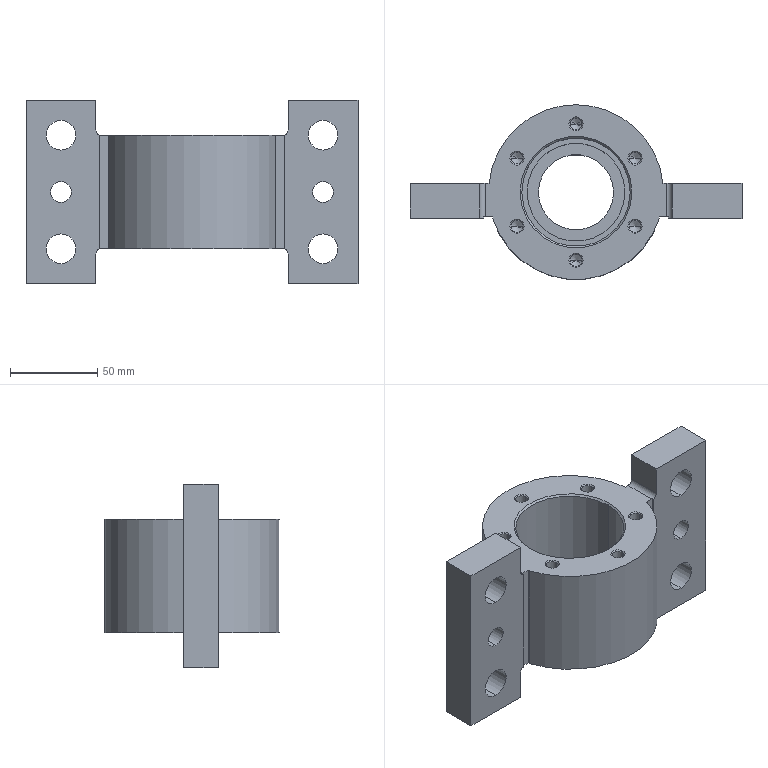Part | SolidWorks | features ICE 7, Attribute 3, HoleWzd 2, Chamfer 1, Extrusion 1 | 1 solid | 134 faces | box 190 x 100 x 105 mm | volume 479131 mm3 | cylinder 56 | cone 50 | plane 28 | commonest cylinder face diameters 5 x12 6.8 x12 17 x8 26 x8 6 x4 12 x4